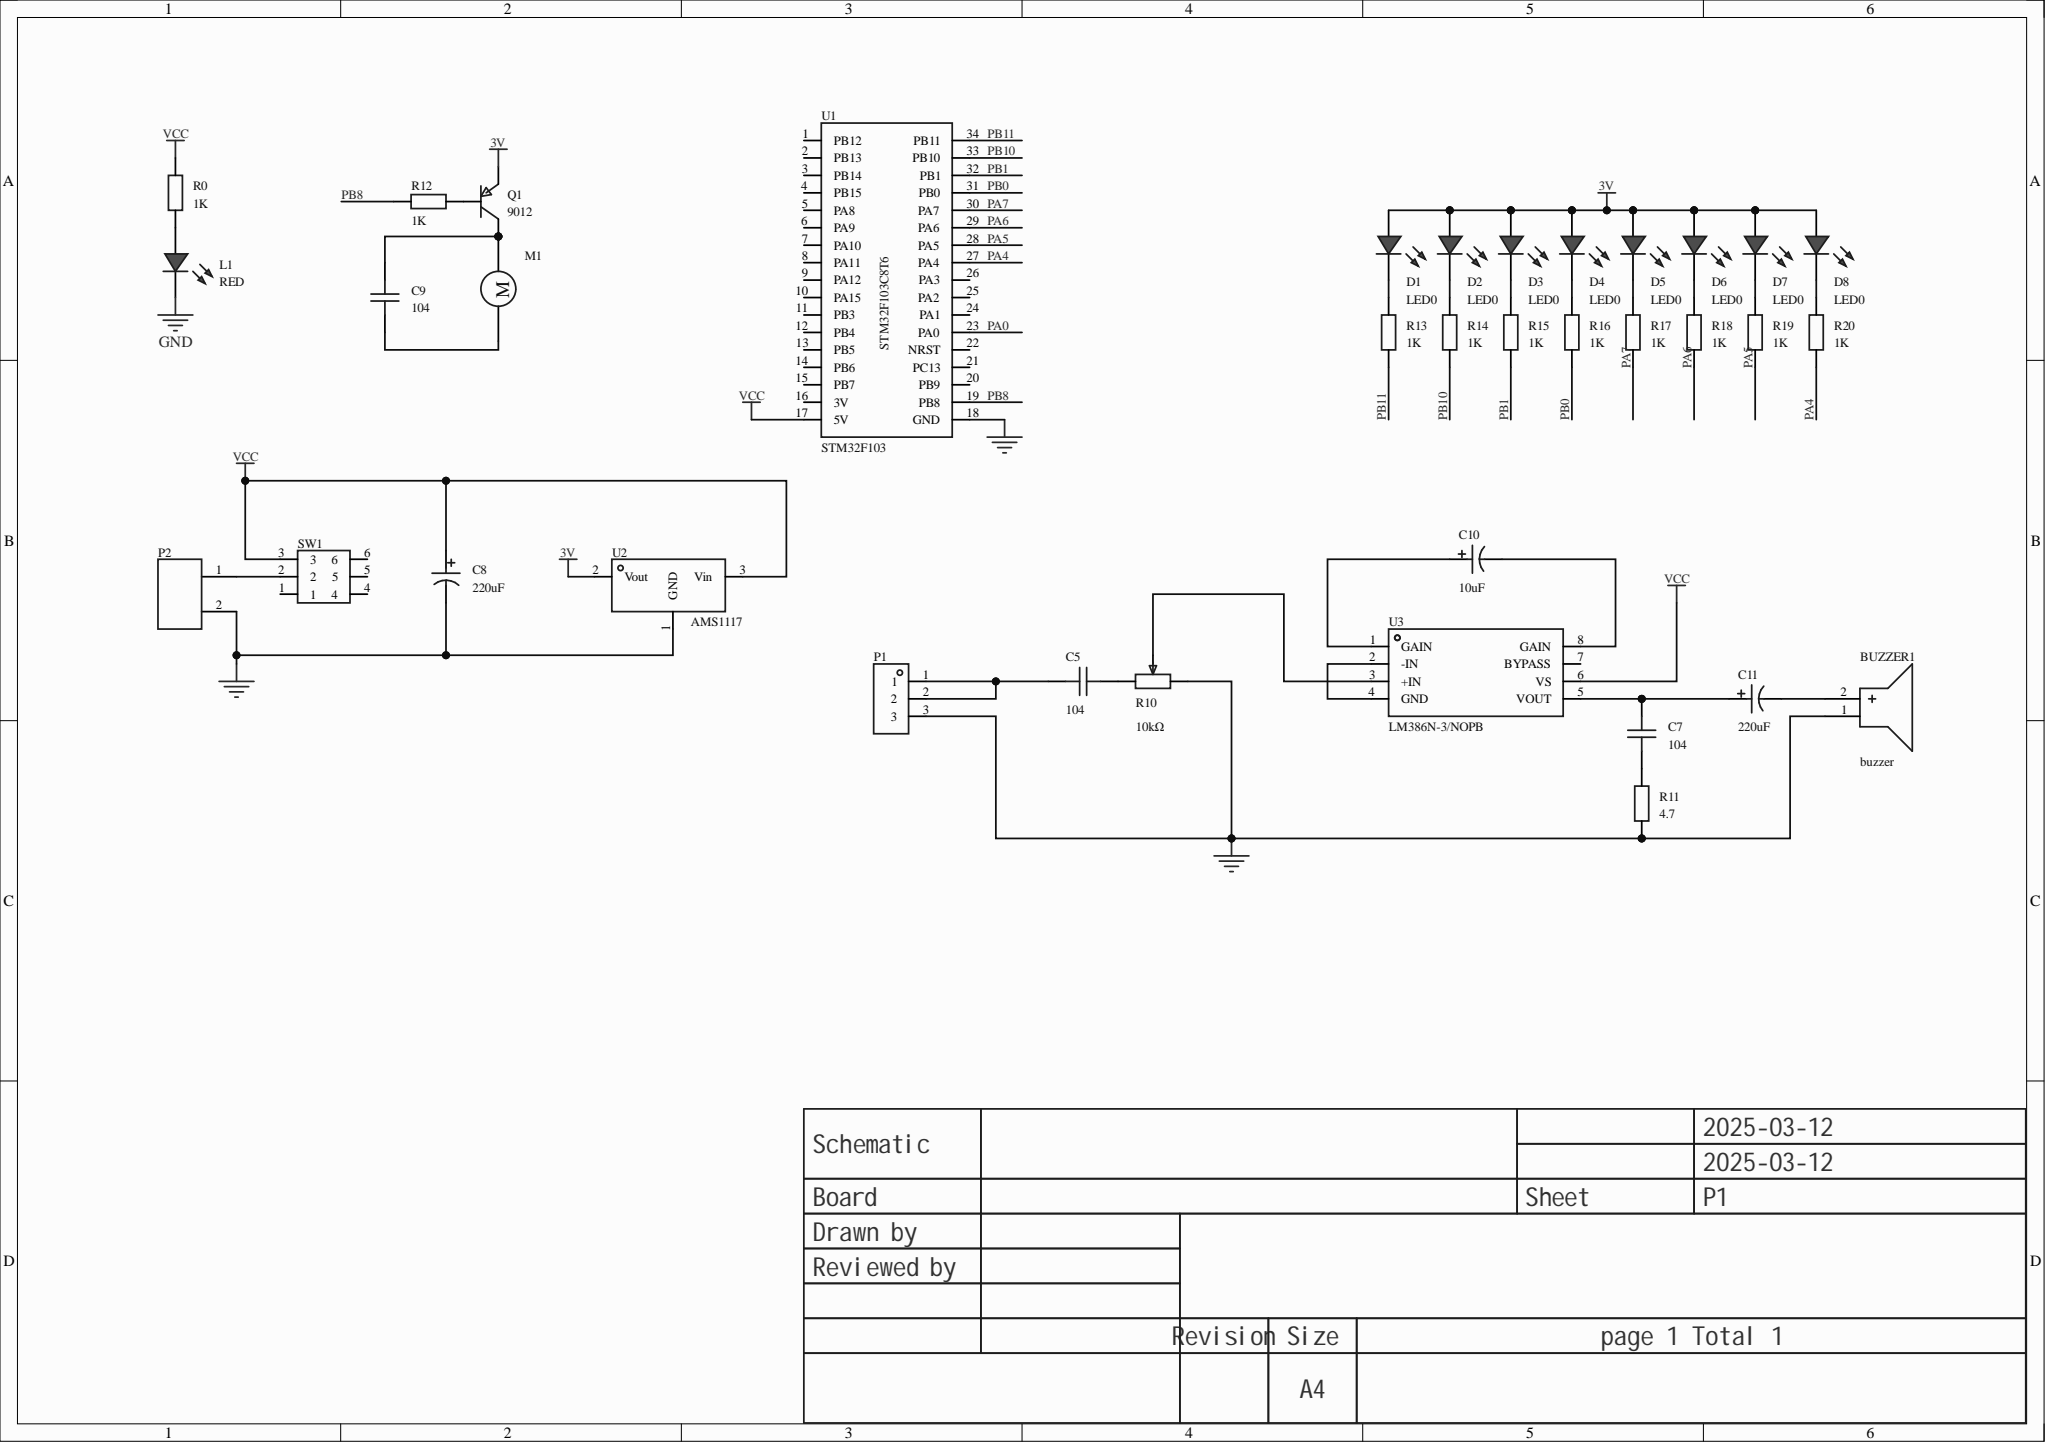Circuit board | Altium Designer | 36 parts | 34 nets
Bill of materials:
Comment,Description,Designator,Footprint,LibRef,Quantity
"buzzer","","BUZZER1","BUZ-TH_BD12.0-P6.00-D0.9-RD","buzzer","1"
"104","","C5, C7, C9","C0805","CAP_0805","3"
"220uF","Capacitance: 220uF; tolerance: ±20%; rated voltage: 10V; ripple current: -; equivalent series resistance: -;","C8, C11","CAP-TH_BD6.3-P2.50-D1.0-FD","EF227M010E05RR0VH4FP0","2"
"10uF","Capacitance: 10uF; tolerance: ±20%; rated voltage: 50V; ripple current: 90mA@100kHz; equivalent series resistance: -;","C10","CAP-TH_BD5.0-P2.00-D0.8-FD","ERM1HM100D11OT","1"
"LED0","","D1, D2, D3, D4, D5, D6, D7, D8","LED_TH-3mm","LED_TH-R_3mm","8"
"RED","","L1","LED_TH-3mm","LED_TH-R_3mm","1"
"Motor","","M1","CONN-TH_2P-P5.08-WJ500V-5.08-2P","Motor","1"
"","","P1","HDR-TH_3P-P2.54-V-M","HDR-M_2.54_1x3P","1"
"DC005","Connector type: DC power socket; mounting: right-angle; contact inner diameter: 2mm; contact outer diameter: 6.3mm; rated current: 500mA; rated voltage: 30V; operating temperature range: -25℃~+70℃;","P2","DC-IN-TH_DC005","DC005","1"
"9012","Transistor type: PNP; collector current (Ic): 500mA; collector-emitter breakdown voltage (Vceo): 25V; power (Pd): 300mW; DC current gain (hFE@Ic,Vce): 120@50mA,1V;","Q1","SOT-23-3_L2.9-W1.3-P1.90-LS2.4-BR","S9012 2T1(RANGE:200-350)","1"
"1K","","R0, R12, R13, R14, R15, R16, R17, R18, R19, R20","R0603","Res_0603","10"
"10kΩ","","R10","R_3296","R_3296","1"
"4.7","","R11","R0603","Res_0603","1"
"Switch","","SW1","SW-TH_SS-12D01-GX","开关","1"
"STM32F103","CPU core: ARM-M3; CPU max frequency: 72MHz; application field: -;","U1","LQFP-48_L7.0-W7.0-P0.50-LS9.0-BL","STM32F103C8T6","1"
"AMS1117","Output type: fixed; operating voltage: -; output voltage: 3.3V; output current: 1A; PSRR: 72dB@(120Hz); output polarity: positive;","U2","SOT-223-3_L6.5-W3.4-P2.30-LS7.0-BR","AMS1117-3.3_C6186","1"
"LM386N-3/NOPB","Amplifier type: class AB amplifier; speaker channels: mono; output power: 700mWx1@8Ω;","U3","DIP-8_L9.8-W6.6-P2.54-LS7.6-BL","LM386N-3/NOPB","1"
Netlist (Protel format):
[
BUZZER1
BUZ-TH_BD12.0-P6.00-D0.9-RD
buzzer



]
[
C5
C0805
104



]
[
C7
C0805
104



]
[
C8
CAP-TH_BD6.3-P2.50-D1.0-FD
220uF



]
[
C9
C0805
104



]
[
C10
CAP-TH_BD5.0-P2.00-D0.8-FD
10uF



]
[
C11
CAP-TH_BD6.3-P2.50-D1.0-FD
220uF



]
[
D1
LED_TH-3mm
LED0



]
[
D2
LED_TH-3mm
LED0



]
[
D3
LED_TH-3mm
LED0



]
[
D4
LED_TH-3mm
LED0



]
[
D5
LED_TH-3mm
LED0



]
[
D6
LED_TH-3mm
LED0



]
[
D7
LED_TH-3mm
LED0



]
[
D8
LED_TH-3mm
LED0



]
[
L1
LED_TH-3mm
RED



]
[
M1
CONN-TH_2P-P5.08-WJ500V-5.08-2P
Motor



]
[
P1
HDR-TH_3P-P2.54-V-M




]
[
P2
DC-IN-TH_DC005
DC005



]
[
Q1
SOT-23-3_L2.9-W1.3-P1.90-LS2.4-BR
9012



]
[
R0
R0603
1K



]
[
R10
R_3296
10kΩ



]
[
R11
R0603
4.7



]
[
R12
R0603
1K



]
[
R13
R0603
1K



]
[
R14
R0603
1K



]
[
R15
R0603
1K



]
[
R16
R0603
1K



]
[
R17
R0603
1K



]
[
R18
R0603
1K



]
[
R19
R0603
1K



]
[
R20
R0603
1K



]
[
SW1
SW-TH_SS-12D01-GX
Switch



]
[
U1
LQFP-48_L7.0-W7.0-P0.50-LS9.0-BL
STM32F103



]
[
U2
SOT-223-3_L6.5-W3.4-P2.30-LS7.0-BR
AMS1117



]
[
U3
DIP-8_L9.8-W6.6-P2.54-LS7.6-BL
LM386N-3/NOPB



]
(
VCC
C8-1
R0-2
SW1-3
U1-17
U2-3
U3-6
)
(
PB11
R13-1
U1-34
)
(
PB10
R14-1
U1-33
)
(
PB8
R12-2
U1-19
)
(
PB1
R15-1
U1-32
)
(
PB0
R16-1
U1-31
)
(
PA7
R17-1
U1-30
)
(
PA6
R18-1
U1-29
)
(
PA5
R19-1
U1-28
)
(
PA4
R20-1
U1-27
)
(
NetU3_2
U3-2
U3-4
)
(
NetR10_2
R10-2
U3-3
)
(
NetQ1_1
Q1-1
R12-1
)
(
NetP2_1
P2-1
SW1-2
)
(
NetL1_1
L1-1
R0-1
)
(
NetD8_2
D8-2
R20-2
)
(
NetD7_2
D7-2
R19-2
)
(
NetD6_2
D6-2
R18-2
)
(
NetD5_2
D5-2
R17-2
)
(
NetD4_2
D4-2
R16-2
)
(
NetD3_2
D3-2
R15-2
)
(
NetD2_2
D2-2
R14-2
)
(
NetD1_2
D1-2
R13-2
)
(
NetC10_2
C10-2
U3-8
)
(
NetC10_1
C10-1
U3-1
)
(
NetC9_2
C9-2
M1-1
Q1-3
)
(
NetC9_1
C9-1
M1-2
)
(
NetC7_2
C7-2
R11-2
)
(
NetC7_1
C7-1
C11-1
U3-5
)
(
NetC5_2
C5-2
P1-1
P1-2
)
(
NetC5_1
C5-1
R10-3
)
(
NetBUZZER1_2
BUZZER1-2
C11-2
)
(
GND
BUZZER1-1
C8-2
L1-2
P1-3
P2-2
R10-1
R11-1
U1-18
U2-1
)
(
3V
D1-1
D2-1
D3-1
D4-1
D5-1
D6-1
D7-1
D8-1
Q1-2
U2-2
)